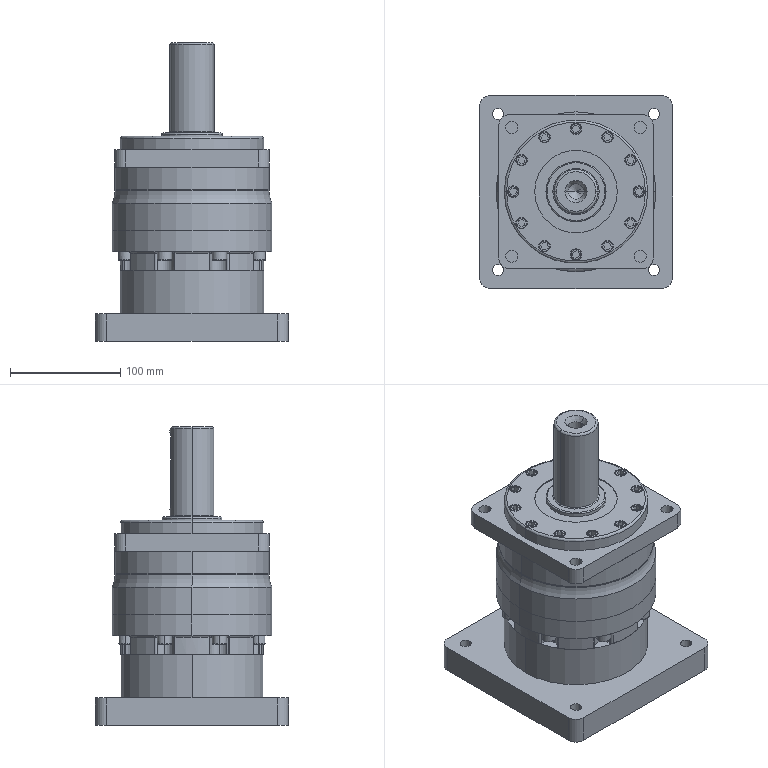Part | SolidWorks | features MBimport 1 | 7 solids | 590 faces | box 175 x 175 x 271 mm | volume 3039277 mm3 | plane 270 | cylinder 197 | torus 103 | spline 16 | cone 4 | commonest cylinder face diameters 10 x24 10.5 x24 4 x20 13 x16 14 x14 130 x13